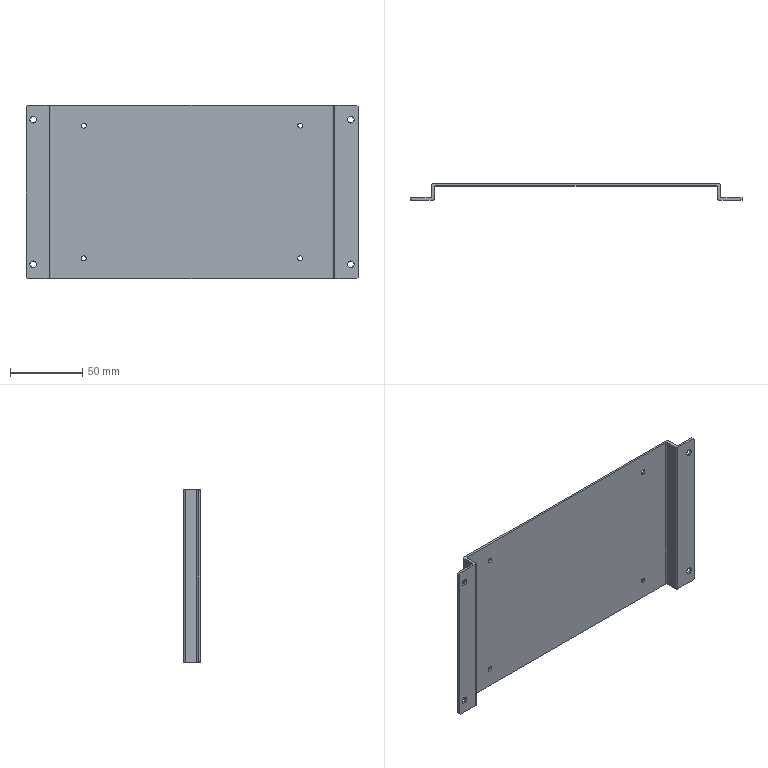Part | NX | 1 solid | 34 faces | box 230 x 11.5 x 120 mm | volume 46044 mm3 | plane 18 | cylinder 16 | commonest cylinder face diameters 2 x8 3.5 x4 4.5 x4
STEP:
#1=CARTESIAN_POINT('',(-41.764,-1.5,119.));
#2=VERTEX_POINT('',#1);
#3=CARTESIAN_POINT('',(-41.764,-1.5,1.));
#4=VERTEX_POINT('',#3);
#5=CARTESIAN_POINT('',(-41.764,-1.5,120.));
#6=DIRECTION('',(0.,0.,-1.));
#7=VECTOR('',#6,1000.);
#8=LINE('',#5,#7);
#9=EDGE_CURVE('',#2,#4,#8,.T.);
#10=ORIENTED_EDGE('',*,*,#9,.F.);
#11=CARTESIAN_POINT('',(-41.764,0.,119.));
#12=VERTEX_POINT('',#11);
#13=CARTESIAN_POINT('',(-41.764,0.,119.));
#14=DIRECTION('',(0.,1.,0.));
#15=VECTOR('',#14,1000.);
#16=LINE('',#13,#15);
#17=EDGE_CURVE('',#2,#12,#16,.T.);
#18=ORIENTED_EDGE('',*,*,#17,.T.);
#19=CARTESIAN_POINT('',(-41.764,0.,1.));
#20=VERTEX_POINT('',#19);
#21=CARTESIAN_POINT('',(-41.764,0.,120.));
#22=DIRECTION('',(0.,0.,-1.));
#23=VECTOR('',#22,1000.);
#24=LINE('',#21,#23);
#25=EDGE_CURVE('',#12,#20,#24,.T.);
#26=ORIENTED_EDGE('',*,*,#25,.T.);
#27=CARTESIAN_POINT('',(-41.764,0.,1.));
#28=DIRECTION('',(0.,-1.,0.));
#29=VECTOR('',#28,1000.);
#30=LINE('',#27,#29);
#31=EDGE_CURVE('',#20,#4,#30,.T.);
#32=ORIENTED_EDGE('',*,*,#31,.T.);
#33=EDGE_LOOP('',(#10,#18,#26,#32));
#34=FACE_BOUND('',#33,.T.);
#35=CARTESIAN_POINT('',(-41.764,0.,120.));
#36=DIRECTION('',(1.,0.,0.));
#37=DIRECTION('',(0.,0.,-1.));
#38=AXIS2_PLACEMENT_3D('',#35,#36,#37);
#39=PLANE('',#38);
#40=ADVANCED_FACE('',(#34),#39,.F.);
#41=CARTESIAN_POINT('',(-36.764,-1.5,12.25));
#42=VERTEX_POINT('',#41);
#43=CARTESIAN_POINT('',(-36.764,-1.5,10.));
#44=DIRECTION('',(0.,1.,0.));
#45=DIRECTION('',(0.,0.,1.));
#46=AXIS2_PLACEMENT_3D('',#43,#44,#45);
#47=CIRCLE('',#46,2.25);
#48=EDGE_CURVE('',#42,#42,#47,.T.);
#49=ORIENTED_EDGE('',*,*,#48,.T.);
#50=EDGE_LOOP('',(#49));
#51=FACE_BOUND('',#50,.T.);
#52=CARTESIAN_POINT('',(-36.764,-1.5,112.25));
#53=VERTEX_POINT('',#52);
#54=CARTESIAN_POINT('',(-36.764,-1.5,110.));
#55=DIRECTION('',(0.,1.,0.));
#56=DIRECTION('',(0.,0.,1.));
#57=AXIS2_PLACEMENT_3D('',#54,#55,#56);
#58=CIRCLE('',#57,2.25);
#59=EDGE_CURVE('',#53,#53,#58,.T.);
#60=ORIENTED_EDGE('',*,*,#59,.T.);
#61=EDGE_LOOP('',(#60));
#62=FACE_BOUND('',#61,.T.);
#63=CARTESIAN_POINT('',(-40.764,-1.5,120.));
#64=VERTEX_POINT('',#63);
#65=CARTESIAN_POINT('',(-25.764,-1.5,120.));
#66=VERTEX_POINT('',#65);
#67=CARTESIAN_POINT('',(-41.764,-1.5,120.));
#68=DIRECTION('',(1.,0.,0.));
#69=VECTOR('',#68,1000.);
#70=LINE('',#67,#69);
#71=EDGE_CURVE('',#64,#66,#70,.T.);
#72=ORIENTED_EDGE('',*,*,#71,.F.);
#73=CARTESIAN_POINT('',(-40.764,-1.5,120.));
#74=DIRECTION('',(-0.7071,0.,-0.7071));
#75=VECTOR('',#74,1000.);
#76=LINE('',#73,#75);
#77=EDGE_CURVE('',#64,#2,#76,.T.);
#78=ORIENTED_EDGE('',*,*,#77,.T.);
#79=ORIENTED_EDGE('',*,*,#9,.T.);
#80=CARTESIAN_POINT('',(-40.764,-1.5,0.));
#81=VERTEX_POINT('',#80);
#82=CARTESIAN_POINT('',(-41.764,-1.5,1.));
#83=DIRECTION('',(-0.7071,0.,0.7071));
#84=VECTOR('',#83,1000.);
#85=LINE('',#82,#84);
#86=EDGE_CURVE('',#4,#81,#85,.F.);
#87=ORIENTED_EDGE('',*,*,#86,.T.);
#88=CARTESIAN_POINT('',(-25.764,-1.5,0.));
#89=VERTEX_POINT('',#88);
#90=CARTESIAN_POINT('',(-41.764,-1.5,0.));
#91=DIRECTION('',(1.,0.,0.));
#92=VECTOR('',#91,1000.);
#93=LINE('',#90,#92);
#94=EDGE_CURVE('',#81,#89,#93,.T.);
#95=ORIENTED_EDGE('',*,*,#94,.T.);
#96=CARTESIAN_POINT('',(-25.764,-1.5,120.));
#97=DIRECTION('',(0.,0.,-1.));
#98=VECTOR('',#97,1000.);
#99=LINE('',#96,#98);
#100=EDGE_CURVE('',#66,#89,#99,.T.);
#101=ORIENTED_EDGE('',*,*,#100,.F.);
#102=EDGE_LOOP('',(#72,#78,#79,#87,#95,#101));
#103=FACE_BOUND('',#102,.T.);
#104=CARTESIAN_POINT('',(-41.764,-1.5,120.));
#105=DIRECTION('',(0.,1.,0.));
#106=DIRECTION('',(0.,0.,1.));
#107=AXIS2_PLACEMENT_3D('',#104,#105,#106);
#108=PLANE('',#107);
#109=ADVANCED_FACE('',(#51,#62,#103),#108,.F.);
#110=CARTESIAN_POINT('',(-24.764,-0.5,0.));
#111=VERTEX_POINT('',#110);
#112=CARTESIAN_POINT('',(-25.764,-0.5,0.));
#113=DIRECTION('',(0.,0.,1.));
#114=DIRECTION('',(1.,0.,0.));
#115=AXIS2_PLACEMENT_3D('',#112,#113,#114);
#116=CIRCLE('',#115,1.);
#117=EDGE_CURVE('',#89,#111,#116,.T.);
#118=ORIENTED_EDGE('',*,*,#117,.T.);
#119=CARTESIAN_POINT('',(-24.764,-0.5,120.));
#120=VERTEX_POINT('',#119);
#121=CARTESIAN_POINT('',(-24.764,-0.5,120.));
#122=DIRECTION('',(0.,0.,-1.));
#123=VECTOR('',#122,1000.);
#124=LINE('',#121,#123);
#125=EDGE_CURVE('',#120,#111,#124,.T.);
#126=ORIENTED_EDGE('',*,*,#125,.F.);
#127=CARTESIAN_POINT('',(-25.764,-0.5,120.));
#128=DIRECTION('',(0.,0.,1.));
#129=DIRECTION('',(1.,0.,0.));
#130=AXIS2_PLACEMENT_3D('',#127,#128,#129);
#131=CIRCLE('',#130,1.);
#132=EDGE_CURVE('',#66,#120,#131,.T.);
#133=ORIENTED_EDGE('',*,*,#132,.F.);
#134=ORIENTED_EDGE('',*,*,#100,.T.);
#135=EDGE_LOOP('',(#118,#126,#133,#134));
#136=FACE_BOUND('',#135,.T.);
#137=CARTESIAN_POINT('',(-25.764,-0.5,120.));
#138=DIRECTION('',(0.,0.,-1.));
#139=DIRECTION('',(-1.,0.,0.));
#140=AXIS2_PLACEMENT_3D('',#137,#138,#139);
#141=CYLINDRICAL_SURFACE('',#140,1.);
#142=ADVANCED_FACE('',(#136),#141,.T.);
#143=CARTESIAN_POINT('',(-24.764,7.5,0.));
#144=VERTEX_POINT('',#143);
#145=CARTESIAN_POINT('',(-24.764,-0.5,0.));
#146=DIRECTION('',(0.,1.,0.));
#147=VECTOR('',#146,1000.);
#148=LINE('',#145,#147);
#149=EDGE_CURVE('',#111,#144,#148,.T.);
#150=ORIENTED_EDGE('',*,*,#149,.T.);
#151=CARTESIAN_POINT('',(-24.764,7.5,120.));
#152=VERTEX_POINT('',#151);
#153=CARTESIAN_POINT('',(-24.764,7.5,120.));
#154=DIRECTION('',(0.,0.,-1.));
#155=VECTOR('',#154,1000.);
#156=LINE('',#153,#155);
#157=EDGE_CURVE('',#152,#144,#156,.T.);
#158=ORIENTED_EDGE('',*,*,#157,.F.);
#159=CARTESIAN_POINT('',(-24.764,-0.5,120.));
#160=DIRECTION('',(0.,1.,0.));
#161=VECTOR('',#160,1000.);
#162=LINE('',#159,#161);
#163=EDGE_CURVE('',#120,#152,#162,.T.);
#164=ORIENTED_EDGE('',*,*,#163,.F.);
#165=ORIENTED_EDGE('',*,*,#125,.T.);
#166=EDGE_LOOP('',(#150,#158,#164,#165));
#167=FACE_BOUND('',#166,.T.);
#168=CARTESIAN_POINT('',(-24.764,-0.5,120.));
#169=DIRECTION('',(-1.,0.,0.));
#170=DIRECTION('',(0.,0.,1.));
#171=AXIS2_PLACEMENT_3D('',#168,#169,#170);
#172=PLANE('',#171);
#173=ADVANCED_FACE('',(#167),#172,.F.);
#174=CARTESIAN_POINT('',(-23.764,8.5,0.));
#175=VERTEX_POINT('',#174);
#176=CARTESIAN_POINT('',(-23.764,7.5,0.));
#177=DIRECTION('',(0.,0.,-1.));
#178=DIRECTION('',(-1.,0.,0.));
#179=AXIS2_PLACEMENT_3D('',#176,#177,#178);
#180=CIRCLE('',#179,1.);
#181=EDGE_CURVE('',#144,#175,#180,.T.);
#182=ORIENTED_EDGE('',*,*,#181,.T.);
#183=CARTESIAN_POINT('',(-23.764,8.5,120.));
#184=VERTEX_POINT('',#183);
#185=CARTESIAN_POINT('',(-23.764,8.5,120.));
#186=DIRECTION('',(0.,0.,-1.));
#187=VECTOR('',#186,1000.);
#188=LINE('',#185,#187);
#189=EDGE_CURVE('',#184,#175,#188,.T.);
#190=ORIENTED_EDGE('',*,*,#189,.F.);
#191=CARTESIAN_POINT('',(-23.764,7.5,120.));
#192=DIRECTION('',(0.,0.,-1.));
#193=DIRECTION('',(-1.,0.,0.));
#194=AXIS2_PLACEMENT_3D('',#191,#192,#193);
#195=CIRCLE('',#194,1.);
#196=EDGE_CURVE('',#152,#184,#195,.T.);
#197=ORIENTED_EDGE('',*,*,#196,.F.);
#198=ORIENTED_EDGE('',*,*,#157,.T.);
#199=EDGE_LOOP('',(#182,#190,#197,#198));
#200=FACE_BOUND('',#199,.T.);
#201=CARTESIAN_POINT('',(-23.764,7.5,120.));
#202=DIRECTION('',(0.,0.,-1.));
#203=DIRECTION('',(-1.,0.,0.));
#204=AXIS2_PLACEMENT_3D('',#201,#202,#203);
#205=CYLINDRICAL_SURFACE('',#204,1.);
#206=ADVANCED_FACE('',(#200),#205,.F.);
#207=CARTESIAN_POINT('',(-3.514,8.5,14.));
#208=VERTEX_POINT('',#207);
#209=CARTESIAN_POINT('',(-1.764,8.5,14.));
#210=DIRECTION('',(0.,1.,0.));
#211=DIRECTION('',(-1.,0.,0.));
#212=AXIS2_PLACEMENT_3D('',#209,#210,#211);
#213=CIRCLE('',#212,1.75);
#214=EDGE_CURVE('',#208,#208,#213,.T.);
#215=ORIENTED_EDGE('',*,*,#214,.T.);
#216=EDGE_LOOP('',(#215));
#217=FACE_BOUND('',#216,.T.);
#218=CARTESIAN_POINT('',(-3.514,8.5,106.));
#219=VERTEX_POINT('',#218);
#220=CARTESIAN_POINT('',(-1.764,8.5,106.));
#221=DIRECTION('',(0.,1.,0.));
#222=DIRECTION('',(-1.,0.,0.));
#223=AXIS2_PLACEMENT_3D('',#220,#221,#222);
#224=CIRCLE('',#223,1.75);
#225=EDGE_CURVE('',#219,#219,#224,.T.);
#226=ORIENTED_EDGE('',*,*,#225,.T.);
#227=EDGE_LOOP('',(#226));
#228=FACE_BOUND('',#227,.T.);
#229=CARTESIAN_POINT('',(146.486,8.5,106.));
#230=VERTEX_POINT('',#229);
#231=CARTESIAN_POINT('',(148.236,8.5,106.));
#232=DIRECTION('',(0.,1.,0.));
#233=DIRECTION('',(-1.,0.,0.));
#234=AXIS2_PLACEMENT_3D('',#231,#232,#233);
#235=CIRCLE('',#234,1.75);
#236=EDGE_CURVE('',#230,#230,#235,.T.);
#237=ORIENTED_EDGE('',*,*,#236,.T.);
#238=EDGE_LOOP('',(#237));
#239=FACE_BOUND('',#238,.T.);
#240=CARTESIAN_POINT('',(146.486,8.5,14.));
#241=VERTEX_POINT('',#240);
#242=CARTESIAN_POINT('',(148.236,8.5,14.));
#243=DIRECTION('',(0.,1.,0.));
#244=DIRECTION('',(-1.,0.,0.));
#245=AXIS2_PLACEMENT_3D('',#242,#243,#244);
#246=CIRCLE('',#245,1.75);
#247=EDGE_CURVE('',#241,#241,#246,.T.);
#248=ORIENTED_EDGE('',*,*,#247,.T.);
#249=EDGE_LOOP('',(#248));
#250=FACE_BOUND('',#249,.T.);
#251=CARTESIAN_POINT('',(170.236,8.5,0.));
#252=VERTEX_POINT('',#251);
#253=CARTESIAN_POINT('',(-23.764,8.5,0.));
#254=DIRECTION('',(1.,0.,0.));
#255=VECTOR('',#254,1000.);
#256=LINE('',#253,#255);
#257=EDGE_CURVE('',#175,#252,#256,.T.);
#258=ORIENTED_EDGE('',*,*,#257,.T.);
#259=CARTESIAN_POINT('',(170.236,8.5,120.));
#260=VERTEX_POINT('',#259);
#261=CARTESIAN_POINT('',(170.236,8.5,120.));
#262=DIRECTION('',(0.,0.,-1.));
#263=VECTOR('',#262,1000.);
#264=LINE('',#261,#263);
#265=EDGE_CURVE('',#260,#252,#264,.T.);
#266=ORIENTED_EDGE('',*,*,#265,.F.);
#267=CARTESIAN_POINT('',(-23.764,8.5,120.));
#268=DIRECTION('',(1.,0.,0.));
#269=VECTOR('',#268,1000.);
#270=LINE('',#267,#269);
#271=EDGE_CURVE('',#184,#260,#270,.T.);
#272=ORIENTED_EDGE('',*,*,#271,.F.);
#273=ORIENTED_EDGE('',*,*,#189,.T.);
#274=EDGE_LOOP('',(#258,#266,#272,#273));
#275=FACE_BOUND('',#274,.T.);
#276=CARTESIAN_POINT('',(-23.764,8.5,120.));
#277=DIRECTION('',(0.,1.,0.));
#278=DIRECTION('',(-1.,0.,0.));
#279=AXIS2_PLACEMENT_3D('',#276,#277,#278);
#280=PLANE('',#279);
#281=ADVANCED_FACE('',(#217,#228,#239,#250,#275),#280,.F.);
#282=CARTESIAN_POINT('',(171.236,7.5,0.));
#283=VERTEX_POINT('',#282);
#284=CARTESIAN_POINT('',(170.236,7.5,0.));
#285=DIRECTION('',(0.,0.,-1.));
#286=DIRECTION('',(-1.,0.,0.));
#287=AXIS2_PLACEMENT_3D('',#284,#285,#286);
#288=CIRCLE('',#287,1.);
#289=EDGE_CURVE('',#252,#283,#288,.T.);
#290=ORIENTED_EDGE('',*,*,#289,.T.);
#291=CARTESIAN_POINT('',(171.236,7.5,120.));
#292=VERTEX_POINT('',#291);
#293=CARTESIAN_POINT('',(171.236,7.5,120.));
#294=DIRECTION('',(0.,0.,-1.));
#295=VECTOR('',#294,1000.);
#296=LINE('',#293,#295);
#297=EDGE_CURVE('',#292,#283,#296,.T.);
#298=ORIENTED_EDGE('',*,*,#297,.F.);
#299=CARTESIAN_POINT('',(170.236,7.5,120.));
#300=DIRECTION('',(0.,0.,-1.));
#301=DIRECTION('',(-1.,0.,0.));
#302=AXIS2_PLACEMENT_3D('',#299,#300,#301);
#303=CIRCLE('',#302,1.);
#304=EDGE_CURVE('',#260,#292,#303,.T.);
#305=ORIENTED_EDGE('',*,*,#304,.F.);
#306=ORIENTED_EDGE('',*,*,#265,.T.);
#307=EDGE_LOOP('',(#290,#298,#305,#306));
#308=FACE_BOUND('',#307,.T.);
#309=CARTESIAN_POINT('',(170.236,7.5,120.));
#310=DIRECTION('',(0.,0.,-1.));
#311=DIRECTION('',(-1.,0.,0.));
#312=AXIS2_PLACEMENT_3D('',#309,#310,#311);
#313=CYLINDRICAL_SURFACE('',#312,1.);
#314=ADVANCED_FACE('',(#308),#313,.F.);
#315=CARTESIAN_POINT('',(171.236,-0.5,0.));
#316=VERTEX_POINT('',#315);
#317=CARTESIAN_POINT('',(171.236,7.5,0.));
#318=DIRECTION('',(0.,-1.,0.));
#319=VECTOR('',#318,1000.);
#320=LINE('',#317,#319);
#321=EDGE_CURVE('',#283,#316,#320,.T.);
#322=ORIENTED_EDGE('',*,*,#321,.T.);
#323=CARTESIAN_POINT('',(171.236,-0.5,120.));
#324=VERTEX_POINT('',#323);
#325=CARTESIAN_POINT('',(171.236,-0.5,120.));
#326=DIRECTION('',(0.,0.,-1.));
#327=VECTOR('',#326,1000.);
#328=LINE('',#325,#327);
#329=EDGE_CURVE('',#324,#316,#328,.T.);
#330=ORIENTED_EDGE('',*,*,#329,.F.);
#331=CARTESIAN_POINT('',(171.236,7.5,120.));
#332=DIRECTION('',(0.,-1.,0.));
#333=VECTOR('',#332,1000.);
#334=LINE('',#331,#333);
#335=EDGE_CURVE('',#292,#324,#334,.T.);
#336=ORIENTED_EDGE('',*,*,#335,.F.);
#337=ORIENTED_EDGE('',*,*,#297,.T.);
#338=EDGE_LOOP('',(#322,#330,#336,#337));
#339=FACE_BOUND('',#338,.T.);
#340=CARTESIAN_POINT('',(171.236,7.5,120.));
#341=DIRECTION('',(1.,0.,0.));
#342=DIRECTION('',(0.,0.,-1.));
#343=AXIS2_PLACEMENT_3D('',#340,#341,#342);
#344=PLANE('',#343);
#345=ADVANCED_FACE('',(#339),#344,.F.);
#346=CARTESIAN_POINT('',(172.236,-1.5,0.));
#347=VERTEX_POINT('',#346);
#348=CARTESIAN_POINT('',(172.236,-0.5,0.));
#349=DIRECTION('',(0.,0.,1.));
#350=DIRECTION('',(1.,0.,0.));
#351=AXIS2_PLACEMENT_3D('',#348,#349,#350);
#352=CIRCLE('',#351,1.);
#353=EDGE_CURVE('',#316,#347,#352,.T.);
#354=ORIENTED_EDGE('',*,*,#353,.T.);
#355=CARTESIAN_POINT('',(172.236,-1.5,120.));
#356=VERTEX_POINT('',#355);
#357=CARTESIAN_POINT('',(172.236,-1.5,120.));
#358=DIRECTION('',(0.,0.,-1.));
#359=VECTOR('',#358,1000.);
#360=LINE('',#357,#359);
#361=EDGE_CURVE('',#356,#347,#360,.T.);
#362=ORIENTED_EDGE('',*,*,#361,.F.);
#363=CARTESIAN_POINT('',(172.236,-0.5,120.));
#364=DIRECTION('',(0.,0.,1.));
#365=DIRECTION('',(1.,0.,0.));
#366=AXIS2_PLACEMENT_3D('',#363,#364,#365);
#367=CIRCLE('',#366,1.);
#368=EDGE_CURVE('',#324,#356,#367,.T.);
#369=ORIENTED_EDGE('',*,*,#368,.F.);
#370=ORIENTED_EDGE('',*,*,#329,.T.);
#371=EDGE_LOOP('',(#354,#362,#369,#370));
#372=FACE_BOUND('',#371,.T.);
#373=CARTESIAN_POINT('',(172.236,-0.5,120.));
#374=DIRECTION('',(0.,0.,-1.));
#375=DIRECTION('',(-1.,0.,0.));
#376=AXIS2_PLACEMENT_3D('',#373,#374,#375);
#377=CYLINDRICAL_SURFACE('',#376,1.);
#378=ADVANCED_FACE('',(#372),#377,.T.);
#379=CARTESIAN_POINT('',(183.236,-1.5,112.25));
#380=VERTEX_POINT('',#379);
#381=CARTESIAN_POINT('',(183.236,-1.5,110.));
#382=DIRECTION('',(0.,1.,0.));
#383=DIRECTION('',(0.,0.,1.));
#384=AXIS2_PLACEMENT_3D('',#381,#382,#383);
#385=CIRCLE('',#384,2.25);
#386=EDGE_CURVE('',#380,#380,#385,.T.);
#387=ORIENTED_EDGE('',*,*,#386,.T.);
#388=EDGE_LOOP('',(#387));
#389=FACE_BOUND('',#388,.T.);
#390=CARTESIAN_POINT('',(183.236,-1.5,12.25));
#391=VERTEX_POINT('',#390);
#392=CARTESIAN_POINT('',(183.236,-1.5,10.));
#393=DIRECTION('',(0.,1.,0.));
#394=DIRECTION('',(0.,0.,1.));
#395=AXIS2_PLACEMENT_3D('',#392,#393,#394);
#396=CIRCLE('',#395,2.25);
#397=EDGE_CURVE('',#391,#391,#396,.T.);
#398=ORIENTED_EDGE('',*,*,#397,.T.);
#399=EDGE_LOOP('',(#398));
#400=FACE_BOUND('',#399,.T.);
#401=CARTESIAN_POINT('',(187.236,-1.5,0.));
#402=VERTEX_POINT('',#401);
#403=CARTESIAN_POINT('',(172.236,-1.5,0.));
#404=DIRECTION('',(1.,0.,0.));
#405=VECTOR('',#404,1000.);
#406=LINE('',#403,#405);
#407=EDGE_CURVE('',#347,#402,#406,.T.);
#408=ORIENTED_EDGE('',*,*,#407,.T.);
#409=CARTESIAN_POINT('',(188.236,-1.5,1.));
#410=VERTEX_POINT('',#409);
#411=CARTESIAN_POINT('',(188.236,-1.5,1.));
#412=DIRECTION('',(-0.7071,0.,-0.7071));
#413=VECTOR('',#412,1000.);
#414=LINE('',#411,#413);
#415=EDGE_CURVE('',#402,#410,#414,.F.);
#416=ORIENTED_EDGE('',*,*,#415,.T.);
#417=CARTESIAN_POINT('',(188.236,-1.5,119.));
#418=VERTEX_POINT('',#417);
#419=CARTESIAN_POINT('',(188.236,-1.5,120.));
#420=DIRECTION('',(0.,0.,-1.));
#421=VECTOR('',#420,1000.);
#422=LINE('',#419,#421);
#423=EDGE_CURVE('',#418,#410,#422,.T.);
#424=ORIENTED_EDGE('',*,*,#423,.F.);
#425=CARTESIAN_POINT('',(187.236,-1.5,120.));
#426=VERTEX_POINT('',#425);
#427=CARTESIAN_POINT('',(187.236,-1.5,120.));
#428=DIRECTION('',(-0.7071,0.,0.7071));
#429=VECTOR('',#428,1000.);
#430=LINE('',#427,#429);
#431=EDGE_CURVE('',#418,#426,#430,.T.);
#432=ORIENTED_EDGE('',*,*,#431,.T.);
#433=CARTESIAN_POINT('',(172.236,-1.5,120.));
#434=DIRECTION('',(1.,0.,0.));
#435=VECTOR('',#434,1000.);
#436=LINE('',#433,#435);
#437=EDGE_CURVE('',#356,#426,#436,.T.);
#438=ORIENTED_EDGE('',*,*,#437,.F.);
#439=ORIENTED_EDGE('',*,*,#361,.T.);
#440=EDGE_LOOP('',(#408,#416,#424,#432,#438,#439));
#441=FACE_BOUND('',#440,.T.);
#442=CARTESIAN_POINT('',(172.236,-1.5,120.));
#443=DIRECTION('',(0.,1.,0.));
#444=DIRECTION('',(0.,0.,1.));
#445=AXIS2_PLACEMENT_3D('',#442,#443,#444);
#446=PLANE('',#445);
#447=ADVANCED_FACE('',(#389,#400,#441),#446,.F.);
#448=ORIENTED_EDGE('',*,*,#423,.T.);
#449=CARTESIAN_POINT('',(188.236,0.,1.));
#450=VERTEX_POINT('',#449);
#451=CARTESIAN_POINT('',(188.236,-1.5,1.));
#452=DIRECTION('',(0.,1.,0.));
#453=VECTOR('',#452,1000.);
#454=LINE('',#451,#453);
#455=EDGE_CURVE('',#410,#450,#454,.T.);
#456=ORIENTED_EDGE('',*,*,#455,.T.);
#457=CARTESIAN_POINT('',(188.236,0.,119.));
#458=VERTEX_POINT('',#457);
#459=CARTESIAN_POINT('',(188.236,0.,120.));
#460=DIRECTION('',(0.,0.,-1.));
#461=VECTOR('',#460,1000.);
#462=LINE('',#459,#461);
#463=EDGE_CURVE('',#458,#450,#462,.T.);
#464=ORIENTED_EDGE('',*,*,#463,.F.);
#465=CARTESIAN_POINT('',(188.236,-1.5,119.));
#466=DIRECTION('',(0.,-1.,0.));
#467=VECTOR('',#466,1000.);
#468=LINE('',#465,#467);
#469=EDGE_CURVE('',#458,#418,#468,.T.);
#470=ORIENTED_EDGE('',*,*,#469,.T.);
#471=EDGE_LOOP('',(#448,#456,#464,#470));
#472=FACE_BOUND('',#471,.T.);
#473=CARTESIAN_POINT('',(188.236,-1.5,120.));
#474=DIRECTION('',(-1.,0.,0.));
#475=DIRECTION('',(0.,0.,1.));
#476=AXIS2_PLACEMENT_3D('',#473,#474,#475);
#477=PLANE('',#476);
#478=ADVANCED_FACE('',(#472),#477,.F.);
#479=CARTESIAN_POINT('',(183.236,0.,112.25));
#480=VERTEX_POINT('',#479);
#481=CARTESIAN_POINT('',(183.236,0.,110.));
#482=DIRECTION('',(0.,1.,0.));
#483=DIRECTION('',(0.,0.,1.));
#484=AXIS2_PLACEMENT_3D('',#481,#482,#483);
#485=CIRCLE('',#484,2.25);
#486=EDGE_CURVE('',#480,#480,#485,.T.);
#487=ORIENTED_EDGE('',*,*,#486,.F.);
#488=EDGE_LOOP('',(#487));
#489=FACE_BOUND('',#488,.T.);
#490=CARTESIAN_POINT('',(183.236,0.,12.25));
#491=VERTEX_POINT('',#490);
#492=CARTESIAN_POINT('',(183.236,0.,10.));
#493=DIRECTION('',(0.,1.,0.));
#494=DIRECTION('',(0.,0.,1.));
#495=AXIS2_PLACEMENT_3D('',#492,#493,#494);
#496=CIRCLE('',#495,2.25);
#497=EDGE_CURVE('',#491,#491,#496,.T.);
#498=ORIENTED_EDGE('',*,*,#497,.F.);
#499=EDGE_LOOP('',(#498));
#500=FACE_BOUND('',#499,.T.);
#501=ORIENTED_EDGE('',*,*,#463,.T.);
#502=CARTESIAN_POINT('',(187.236,0.,0.));
#503=VERTEX_POINT('',#502);
#504=CARTESIAN_POINT('',(188.236,0.,1.));
#505=DIRECTION('',(0.7071,0.,0.7071));
#506=VECTOR('',#505,1000.);
#507=LINE('',#504,#506);
#508=EDGE_CURVE('',#450,#503,#507,.F.);
#509=ORIENTED_EDGE('',*,*,#508,.T.);
#510=CARTESIAN_POINT('',(174.236,0.,0.));
#511=VERTEX_POINT('',#510);
#512=CARTESIAN_POINT('',(174.236,0.,0.));
#513=DIRECTION('',(-1.,0.,0.));
#514=VECTOR('',#513,1000.);
#515=LINE('',#512,#514);
#516=EDGE_CURVE('',#503,#511,#515,.T.);
#517=ORIENTED_EDGE('',*,*,#516,.T.);
#518=CARTESIAN_POINT('',(174.236,0.,120.));
#519=VERTEX_POINT('',#518);
#520=CARTESIAN_POINT('',(174.236,0.,120.));
#521=DIRECTION('',(0.,0.,-1.));
#522=VECTOR('',#521,1000.);
#523=LINE('',#520,#522);
#524=EDGE_CURVE('',#519,#511,#523,.T.);
#525=ORIENTED_EDGE('',*,*,#524,.F.);
#526=CARTESIAN_POINT('',(187.236,0.,120.));
#527=VERTEX_POINT('',#526);
#528=CARTESIAN_POINT('',(174.236,0.,120.));
#529=DIRECTION('',(-1.,0.,0.));
#530=VECTOR('',#529,1000.);
#531=LINE('',#528,#530);
#532=EDGE_CURVE('',#527,#519,#531,.T.);
#533=ORIENTED_EDGE('',*,*,#532,.F.);
#534=CARTESIAN_POINT('',(187.236,0.,120.));
#535=DIRECTION('',(0.7071,0.,-0.7071));
#536=VECTOR('',#535,1000.);
#537=LINE('',#534,#536);
#538=EDGE_CURVE('',#527,#458,#537,.T.);
#539=ORIENTED_EDGE('',*,*,#538,.T.);
#540=EDGE_LOOP('',(#501,#509,#517,#525,#533,#539));
#541=FACE_BOUND('',#540,.T.);
#542=CARTESIAN_POINT('',(174.236,0.,120.));
#543=DIRECTION('',(0.,-1.,0.));
#544=DIRECTION('',(0.,0.,-1.));
#545=AXIS2_PLACEMENT_3D('',#542,#543,#544);
#546=PLANE('',#545);
#547=ADVANCED_FACE('',(#489,#500,#541),#546,.F.);
#548=CARTESIAN_POINT('',(173.236,1.,0.));
#549=VERTEX_POINT('',#548);
#550=CARTESIAN_POINT('',(174.236,1.,0.));
#551=DIRECTION('',(0.,0.,-1.));
#552=DIRECTION('',(1.,0.,0.));
#553=AXIS2_PLACEMENT_3D('',#550,#551,#552);
#554=CIRCLE('',#553,1.);
#555=EDGE_CURVE('',#511,#549,#554,.T.);
#556=ORIENTED_EDGE('',*,*,#555,.T.);
#557=CARTESIAN_POINT('',(173.236,1.,120.));
#558=VERTEX_POINT('',#557);
#559=CARTESIAN_POINT('',(173.236,1.,120.));
#560=DIRECTION('',(0.,0.,-1.));
#561=VECTOR('',#560,1000.);
#562=LINE('',#559,#561);
#563=EDGE_CURVE('',#558,#549,#562,.T.);
#564=ORIENTED_EDGE('',*,*,#563,.F.);
#565=CARTESIAN_POINT('',(174.236,1.,120.));
#566=DIRECTION('',(0.,0.,-1.));
#567=DIRECTION('',(1.,0.,0.));
#568=AXIS2_PLACEMENT_3D('',#565,#566,#567);
#569=CIRCLE('',#568,1.);
#570=EDGE_CURVE('',#519,#558,#569,.T.);
#571=ORIENTED_EDGE('',*,*,#570,.F.);
#572=ORIENTED_EDGE('',*,*,#524,.T.);
#573=EDGE_LOOP('',(#556,#564,#571,#572));
#574=FACE_BOUND('',#573,.T.);
#575=CARTESIAN_POINT('',(174.236,1.,120.));
#576=DIRECTION('',(0.,0.,-1.));
#577=DIRECTION('',(-1.,0.,0.));
#578=AXIS2_PLACEMENT_3D('',#575,#576,#577);
#579=CYLINDRICAL_SURFACE('',#578,1.);
#580=ADVANCED_FACE('',(#574),#579,.F.);
#581=CARTESIAN_POINT('',(173.236,9.,0.));
#582=VERTEX_POINT('',#581);
#583=CARTESIAN_POINT('',(173.236,9.,0.));
#584=DIRECTION('',(0.,1.,0.));
#585=VECTOR('',#584,1000.);
#586=LINE('',#583,#585);
#587=EDGE_CURVE('',#549,#582,#586,.T.);
#588=ORIENTED_EDGE('',*,*,#587,.T.);
#589=CARTESIAN_POINT('',(173.236,9.,120.));
#590=VERTEX_POINT('',#589);
#591=CARTESIAN_POINT('',(173.236,9.,120.));
#592=DIRECTION('',(0.,0.,-1.));
#593=VECTOR('',#592,1000.);
#594=LINE('',#591,#593);
#595=EDGE_CURVE('',#590,#582,#594,.T.);
#596=ORIENTED_EDGE('',*,*,#595,.F.);
#597=CARTESIAN_POINT('',(173.236,9.,120.));
#598=DIRECTION('',(0.,1.,0.));
#599=VECTOR('',#598,1000.);
#600=LINE('',#597,#599);
#601=EDGE_CURVE('',#558,#590,#600,.T.);
#602=ORIENTED_EDGE('',*,*,#601,.F.);
#603=ORIENTED_EDGE('',*,*,#563,.T.);
#604=EDGE_LOOP('',(#588,#596,#602,#603));
#605=FACE_BOUND('',#604,.T.);
#606=CARTESIAN_POINT('',(173.236,9.,120.));
#607=DIRECTION('',(-1.,0.,0.));
#608=DIRECTION('',(0.,0.,1.));
#609=AXIS2_PLACEMENT_3D('',#606,#607,#608);
#610=PLANE('',#609);
#611=ADVANCED_FACE('',(#605),#610,.F.);
#612=CARTESIAN_POINT('',(172.236,10.,0.));
#613=VERTEX_POINT('',#612);
#614=CARTESIAN_POINT('',(172.236,9.,0.));
#615=DIRECTION('',(0.,0.,1.));
#616=DIRECTION('',(-1.,0.,0.));
#617=AXIS2_PLACEMENT_3D('',#614,#615,#616);
#618=CIRCLE('',#617,1.);
#619=EDGE_CURVE('',#582,#613,#618,.T.);
#620=ORIENTED_EDGE('',*,*,#619,.T.);
#621=CARTESIAN_POINT('',(172.236,10.,120.));
#622=VERTEX_POINT('',#621);
#623=CARTESIAN_POINT('',(172.236,10.,120.));
#624=DIRECTION('',(0.,0.,-1.));
#625=VECTOR('',#624,1000.);
#626=LINE('',#623,#625);
#627=EDGE_CURVE('',#622,#613,#626,.T.);
#628=ORIENTED_EDGE('',*,*,#627,.F.);
#629=CARTESIAN_POINT('',(172.236,9.,120.));
#630=DIRECTION('',(0.,0.,1.));
#631=DIRECTION('',(-1.,0.,0.));
#632=AXIS2_PLACEMENT_3D('',#629,#630,#631);
#633=CIRCLE('',#632,1.);
#634=EDGE_CURVE('',#590,#622,#633,.T.);
#635=ORIENTED_EDGE('',*,*,#634,.F.);
#636=ORIENTED_EDGE('',*,*,#595,.T.);
#637=EDGE_LOOP('',(#620,#628,#635,#636));
#638=FACE_BOUND('',#637,.T.);
#639=CARTESIAN_POINT('',(172.236,9.,120.));
#640=DIRECTION('',(0.,0.,-1.));
#641=DIRECTION('',(-1.,0.,0.));
#642=AXIS2_PLACEMENT_3D('',#639,#640,#641);
#643=CYLINDRICAL_SURFACE('',#642,1.);
#644=ADVANCED_FACE('',(#638),#643,.T.);
#645=CARTESIAN_POINT('',(-1.764,10.,15.75));
#646=VERTEX_POINT('',#645);
#647=CARTESIAN_POINT('',(-1.764,10.,14.));
#648=DIRECTION('',(0.,1.,0.));
#649=DIRECTION('',(0.,0.,1.));
#650=AXIS2_PLACEMENT_3D('',#647,#648,#649);
#651=CIRCLE('',#650,1.75);
#652=EDGE_CURVE('',#646,#646,#651,.T.);
#653=ORIENTED_EDGE('',*,*,#652,.F.);
#654=EDGE_LOOP('',(#653));
#655=FACE_BOUND('',#654,.T.);
#656=CARTESIAN_POINT('',(-1.764,10.,107.75));
#657=VERTEX_POINT('',#656);
#658=CARTESIAN_POINT('',(-1.764,10.,106.));
#659=DIRECTION('',(0.,1.,0.));
#660=DIRECTION('',(0.,0.,1.));
#661=AXIS2_PLACEMENT_3D('',#658,#659,#660);
#662=CIRCLE('',#661,1.75);
#663=EDGE_CURVE('',#657,#657,#662,.T.);
#664=ORIENTED_EDGE('',*,*,#663,.F.);
#665=EDGE_LOOP('',(#664));
#666=FACE_BOUND('',#665,.T.);
#667=CARTESIAN_POINT('',(148.236,10.,107.75));
#668=VERTEX_POINT('',#667);
#669=CARTESIAN_POINT('',(148.236,10.,106.));
#670=DIRECTION('',(0.,1.,0.));
#671=DIRECTION('',(0.,0.,1.));
#672=AXIS2_PLACEMENT_3D('',#669,#670,#671);
#673=CIRCLE('',#672,1.75);
#674=EDGE_CURVE('',#668,#668,#673,.T.);
#675=ORIENTED_EDGE('',*,*,#674,.F.);
#676=EDGE_LOOP('',(#675));
#677=FACE_BOUND('',#676,.T.);
#678=CARTESIAN_POINT('',(148.236,10.,15.75));
#679=VERTEX_POINT('',#678);
#680=CARTESIAN_POINT('',(148.236,10.,14.));
#681=DIRECTION('',(0.,1.,0.));
#682=DIRECTION('',(0.,0.,1.));
#683=AXIS2_PLACEMENT_3D('',#680,#681,#682);
#684=CIRCLE('',#683,1.75);
#685=EDGE_CURVE('',#679,#679,#684,.T.);
#686=ORIENTED_EDGE('',*,*,#685,.F.);
#687=EDGE_LOOP('',(#686));
#688=FACE_BOUND('',#687,.T.);
#689=CARTESIAN_POINT('',(-25.764,10.,0.));
#690=VERTEX_POINT('',#689);
#691=CARTESIAN_POINT('',(-25.764,10.,0.));
#692=DIRECTION('',(-1.,0.,0.));
#693=VECTOR('',#692,1000.);
#694=LINE('',#691,#693);
#695=EDGE_CURVE('',#613,#690,#694,.T.);
#696=ORIENTED_EDGE('',*,*,#695,.T.);
#697=CARTESIAN_POINT('',(-25.764,10.,120.));
#698=VERTEX_POINT('',#697);
#699=CARTESIAN_POINT('',(-25.764,10.,120.));
#700=DIRECTION('',(0.,0.,-1.));
#701=VECTOR('',#700,1000.);
#702=LINE('',#699,#701);
#703=EDGE_CURVE('',#698,#690,#702,.T.);
#704=ORIENTED_EDGE('',*,*,#703,.F.);
#705=CARTESIAN_POINT('',(-25.764,10.,120.));
#706=DIRECTION('',(-1.,0.,0.));
#707=VECTOR('',#706,1000.);
#708=LINE('',#705,#707);
#709=EDGE_CURVE('',#622,#698,#708,.T.);
#710=ORIENTED_EDGE('',*,*,#709,.F.);
#711=ORIENTED_EDGE('',*,*,#627,.T.);
#712=EDGE_LOOP('',(#696,#704,#710,#711));
#713=FACE_BOUND('',#712,.T.);
#714=CARTESIAN_POINT('',(-25.764,10.,120.));
#715=DIRECTION('',(0.,-1.,0.));
#716=DIRECTION('',(0.,0.,-1.));
#717=AXIS2_PLACEMENT_3D('',#714,#715,#716);
#718=PLANE('',#717);
#719=ADVANCED_FACE('',(#655,#666,#677,#688,#713),#718,.F.);
#720=CARTESIAN_POINT('',(-26.764,9.,0.));
#721=VERTEX_POINT('',#720);
#722=CARTESIAN_POINT('',(-25.764,9.,0.));
#723=DIRECTION('',(0.,0.,1.));
#724=DIRECTION('',(-1.,0.,0.));
#725=AXIS2_PLACEMENT_3D('',#722,#723,#724);
#726=CIRCLE('',#725,1.);
#727=EDGE_CURVE('',#690,#721,#726,.T.);
#728=ORIENTED_EDGE('',*,*,#727,.T.);
#729=CARTESIAN_POINT('',(-26.764,9.,120.));
#730=VERTEX_POINT('',#729);
#731=CARTESIAN_POINT('',(-26.764,9.,120.));
#732=DIRECTION('',(0.,0.,-1.));
#733=VECTOR('',#732,1000.);
#734=LINE('',#731,#733);
#735=EDGE_CURVE('',#730,#721,#734,.T.);
#736=ORIENTED_EDGE('',*,*,#735,.F.);
#737=CARTESIAN_POINT('',(-25.764,9.,120.));
#738=DIRECTION('',(0.,0.,1.));
#739=DIRECTION('',(-1.,0.,0.));
#740=AXIS2_PLACEMENT_3D('',#737,#738,#739);
#741=CIRCLE('',#740,1.);
#742=EDGE_CURVE('',#698,#730,#741,.T.);
#743=ORIENTED_EDGE('',*,*,#742,.F.);
#744=ORIENTED_EDGE('',*,*,#703,.T.);
#745=EDGE_LOOP('',(#728,#736,#743,#744));
#746=FACE_BOUND('',#745,.T.);
#747=CARTESIAN_POINT('',(-25.764,9.,120.));
#748=DIRECTION('',(0.,0.,-1.));
#749=DIRECTION('',(-1.,0.,0.));
#750=AXIS2_PLACEMENT_3D('',#747,#748,#749);
#751=CYLINDRICAL_SURFACE('',#750,1.);
#752=ADVANCED_FACE('',(#746),#751,.T.);
#753=CARTESIAN_POINT('',(-26.764,1.,0.));
#754=VERTEX_POINT('',#753);
#755=CARTESIAN_POINT('',(-26.764,1.,0.));
#756=DIRECTION('',(0.,-1.,0.));
#757=VECTOR('',#756,1000.);
#758=LINE('',#755,#757);
#759=EDGE_CURVE('',#721,#754,#758,.T.);
#760=ORIENTED_EDGE('',*,*,#759,.T.);
#761=CARTESIAN_POINT('',(-26.764,1.,120.));
#762=VERTEX_POINT('',#761);
#763=CARTESIAN_POINT('',(-26.764,1.,120.));
#764=DIRECTION('',(0.,0.,-1.));
#765=VECTOR('',#764,1000.);
#766=LINE('',#763,#765);
#767=EDGE_CURVE('',#762,#754,#766,.T.);
#768=ORIENTED_EDGE('',*,*,#767,.F.);
#769=CARTESIAN_POINT('',(-26.764,1.,120.));
#770=DIRECTION('',(0.,-1.,0.));
#771=VECTOR('',#770,1000.);
#772=LINE('',#769,#771);
#773=EDGE_CURVE('',#730,#762,#772,.T.);
#774=ORIENTED_EDGE('',*,*,#773,.F.);
#775=ORIENTED_EDGE('',*,*,#735,.T.);
#776=EDGE_LOOP('',(#760,#768,#774,#775));
#777=FACE_BOUND('',#776,.T.);
#778=CARTESIAN_POINT('',(-26.764,1.,120.));
#779=DIRECTION('',(1.,0.,0.));
#780=DIRECTION('',(0.,0.,-1.));
#781=AXIS2_PLACEMENT_3D('',#778,#779,#780);
#782=PLANE('',#781);
#783=ADVANCED_FACE('',(#777),#782,.F.);
#784=CARTESIAN_POINT('',(-27.764,0.,0.));
#785=VERTEX_POINT('',#784);
#786=CARTESIAN_POINT('',(-27.764,1.,0.));
#787=DIRECTION('',(0.,0.,-1.));
#788=DIRECTION('',(1.,0.,0.));
#789=AXIS2_PLACEMENT_3D('',#786,#787,#788);
#790=CIRCLE('',#789,1.);
#791=EDGE_CURVE('',#754,#785,#790,.T.);
#792=ORIENTED_EDGE('',*,*,#791,.T.);
#793=CARTESIAN_POINT('',(-27.764,0.,120.));
#794=VERTEX_POINT('',#793);
#795=CARTESIAN_POINT('',(-27.764,0.,120.));
#796=DIRECTION('',(0.,0.,-1.));
#797=VECTOR('',#796,1000.);
#798=LINE('',#795,#797);
#799=EDGE_CURVE('',#794,#785,#798,.T.);
#800=ORIENTED_EDGE('',*,*,#799,.F.);
#801=CARTESIAN_POINT('',(-27.764,1.,120.));
#802=DIRECTION('',(0.,0.,-1.));
#803=DIRECTION('',(1.,0.,0.));
#804=AXIS2_PLACEMENT_3D('',#801,#802,#803);
#805=CIRCLE('',#804,1.);
#806=EDGE_CURVE('',#762,#794,#805,.T.);
#807=ORIENTED_EDGE('',*,*,#806,.F.);
#808=ORIENTED_EDGE('',*,*,#767,.T.);
#809=EDGE_LOOP('',(#792,#800,#807,#808));
#810=FACE_BOUND('',#809,.T.);
#811=CARTESIAN_POINT('',(-27.764,1.,120.));
#812=DIRECTION('',(0.,0.,-1.));
#813=DIRECTION('',(-1.,0.,0.));
#814=AXIS2_PLACEMENT_3D('',#811,#812,#813);
#815=CYLINDRICAL_SURFACE('',#814,1.);
#816=ADVANCED_FACE('',(#810),#815,.F.);
#817=CARTESIAN_POINT('',(-36.764,0.,12.25));
#818=VERTEX_POINT('',#817);
#819=CARTESIAN_POINT('',(-36.764,0.,10.));
#820=DIRECTION('',(0.,1.,0.));
#821=DIRECTION('',(0.,0.,1.));
#822=AXIS2_PLACEMENT_3D('',#819,#820,#821);
#823=CIRCLE('',#822,2.25);
#824=EDGE_CURVE('',#818,#818,#823,.T.);
#825=ORIENTED_EDGE('',*,*,#824,.F.);
#826=EDGE_LOOP('',(#825));
#827=FACE_BOUND('',#826,.T.);
#828=CARTESIAN_POINT('',(-36.764,0.,112.25));
#829=VERTEX_POINT('',#828);
#830=CARTESIAN_POINT('',(-36.764,0.,110.));
#831=DIRECTION('',(0.,1.,0.));
#832=DIRECTION('',(0.,0.,1.));
#833=AXIS2_PLACEMENT_3D('',#830,#831,#832);
#834=CIRCLE('',#833,2.25);
#835=EDGE_CURVE('',#829,#829,#834,.T.);
#836=ORIENTED_EDGE('',*,*,#835,.F.);
#837=EDGE_LOOP('',(#836));
#838=FACE_BOUND('',#837,.T.);
#839=ORIENTED_EDGE('',*,*,#25,.F.);
#840=CARTESIAN_POINT('',(-40.764,0.,120.));
#841=VERTEX_POINT('',#840);
#842=CARTESIAN_POINT('',(-40.764,0.,120.));
#843=DIRECTION('',(0.7071,0.,0.7071));
#844=VECTOR('',#843,1000.);
#845=LINE('',#842,#844);
#846=EDGE_CURVE('',#12,#841,#845,.T.);
#847=ORIENTED_EDGE('',*,*,#846,.T.);
#848=CARTESIAN_POINT('',(-41.764,0.,120.));
#849=DIRECTION('',(-1.,0.,0.));
#850=VECTOR('',#849,1000.);
#851=LINE('',#848,#850);
#852=EDGE_CURVE('',#794,#841,#851,.T.);
#853=ORIENTED_EDGE('',*,*,#852,.F.);
#854=ORIENTED_EDGE('',*,*,#799,.T.);
#855=CARTESIAN_POINT('',(-40.764,0.,0.));
#856=VERTEX_POINT('',#855);
#857=CARTESIAN_POINT('',(-41.764,0.,0.));
#858=DIRECTION('',(-1.,0.,0.));
#859=VECTOR('',#858,1000.);
#860=LINE('',#857,#859);
#861=EDGE_CURVE('',#785,#856,#860,.T.);
#862=ORIENTED_EDGE('',*,*,#861,.T.);
#863=CARTESIAN_POINT('',(-41.764,0.,1.));
#864=DIRECTION('',(0.7071,0.,-0.7071));
#865=VECTOR('',#864,1000.);
#866=LINE('',#863,#865);
#867=EDGE_CURVE('',#856,#20,#866,.F.);
#868=ORIENTED_EDGE('',*,*,#867,.T.);
#869=EDGE_LOOP('',(#839,#847,#853,#854,#862,#868));
#870=FACE_BOUND('',#869,.T.);
#871=CARTESIAN_POINT('',(-41.764,0.,120.));
#872=DIRECTION('',(0.,-1.,0.));
#873=DIRECTION('',(0.,0.,-1.));
#874=AXIS2_PLACEMENT_3D('',#871,#872,#873);
#875=PLANE('',#874);
#876=ADVANCED_FACE('',(#827,#838,#870),#875,.F.);
#877=ORIENTED_EDGE('',*,*,#437,.T.);
#878=CARTESIAN_POINT('',(187.236,0.,120.));
#879=DIRECTION('',(0.,1.,0.));
#880=VECTOR('',#879,1000.);
#881=LINE('',#878,#880);
#882=EDGE_CURVE('',#426,#527,#881,.T.);
#883=ORIENTED_EDGE('',*,*,#882,.T.);
#884=ORIENTED_EDGE('',*,*,#532,.T.);
#885=ORIENTED_EDGE('',*,*,#570,.T.);
#886=ORIENTED_EDGE('',*,*,#601,.T.);
#887=ORIENTED_EDGE('',*,*,#634,.T.);
#888=ORIENTED_EDGE('',*,*,#709,.T.);
#889=ORIENTED_EDGE('',*,*,#742,.T.);
#890=ORIENTED_EDGE('',*,*,#773,.T.);
#891=ORIENTED_EDGE('',*,*,#806,.T.);
#892=ORIENTED_EDGE('',*,*,#852,.T.);
#893=CARTESIAN_POINT('',(-40.764,-1.5,120.));
#894=DIRECTION('',(0.,-1.,0.));
#895=VECTOR('',#894,1000.);
#896=LINE('',#893,#895);
#897=EDGE_CURVE('',#841,#64,#896,.T.);
#898=ORIENTED_EDGE('',*,*,#897,.T.);
#899=ORIENTED_EDGE('',*,*,#71,.T.);
#900=ORIENTED_EDGE('',*,*,#132,.T.);
#901=ORIENTED_EDGE('',*,*,#163,.T.);
#902=ORIENTED_EDGE('',*,*,#196,.T.);
#903=ORIENTED_EDGE('',*,*,#271,.T.);
#904=ORIENTED_EDGE('',*,*,#304,.T.);
#905=ORIENTED_EDGE('',*,*,#335,.T.);
#906=ORIENTED_EDGE('',*,*,#368,.T.);
#907=EDGE_LOOP('',(#877,#883,#884,#885,#886,#887,#888,#889,#890,#891,#892,#898,#899,#900,#901,#902,#903,#904,#905,#906));
#908=FACE_BOUND('',#907,.T.);
#909=CARTESIAN_POINT('',(-25.764,-0.5,120.));
#910=DIRECTION('',(0.,0.,1.));
#911=DIRECTION('',(1.,0.,0.));
#912=AXIS2_PLACEMENT_3D('',#909,#910,#911);
#913=PLANE('',#912);
#914=ADVANCED_FACE('',(#908),#913,.T.);
#915=ORIENTED_EDGE('',*,*,#516,.F.);
#916=CARTESIAN_POINT('',(187.236,-0.5,0.));
#917=DIRECTION('',(0.,-1.,0.));
#918=VECTOR('',#917,1000.);
#919=LINE('',#916,#918);
#920=EDGE_CURVE('',#503,#402,#919,.T.);
#921=ORIENTED_EDGE('',*,*,#920,.T.);
#922=ORIENTED_EDGE('',*,*,#407,.F.);
#923=ORIENTED_EDGE('',*,*,#353,.F.);
#924=ORIENTED_EDGE('',*,*,#321,.F.);
#925=ORIENTED_EDGE('',*,*,#289,.F.);
#926=ORIENTED_EDGE('',*,*,#257,.F.);
#927=ORIENTED_EDGE('',*,*,#181,.F.);
#928=ORIENTED_EDGE('',*,*,#149,.F.);
#929=ORIENTED_EDGE('',*,*,#117,.F.);
#930=ORIENTED_EDGE('',*,*,#94,.F.);
#931=CARTESIAN_POINT('',(-40.764,-0.5,0.));
#932=DIRECTION('',(0.,1.,0.));
#933=VECTOR('',#932,1000.);
#934=LINE('',#931,#933);
#935=EDGE_CURVE('',#81,#856,#934,.T.);
#936=ORIENTED_EDGE('',*,*,#935,.T.);
#937=ORIENTED_EDGE('',*,*,#861,.F.);
#938=ORIENTED_EDGE('',*,*,#791,.F.);
#939=ORIENTED_EDGE('',*,*,#759,.F.);
#940=ORIENTED_EDGE('',*,*,#727,.F.);
#941=ORIENTED_EDGE('',*,*,#695,.F.);
#942=ORIENTED_EDGE('',*,*,#619,.F.);
#943=ORIENTED_EDGE('',*,*,#587,.F.);
#944=ORIENTED_EDGE('',*,*,#555,.F.);
#945=EDGE_LOOP('',(#915,#921,#922,#923,#924,#925,#926,#927,#928,#929,#930,#936,#937,#938,#939,#940,#941,#942,#943,#944));
#946=FACE_BOUND('',#945,.T.);
#947=CARTESIAN_POINT('',(-25.764,-0.5,0.));
#948=DIRECTION('',(0.,0.,1.));
#949=DIRECTION('',(1.,0.,0.));
#950=AXIS2_PLACEMENT_3D('',#947,#948,#949);
#951=PLANE('',#950);
#952=ADVANCED_FACE('',(#946),#951,.F.);
#953=ORIENTED_EDGE('',*,*,#397,.F.);
#954=EDGE_LOOP('',(#953));
#955=FACE_BOUND('',#954,.T.);
#956=ORIENTED_EDGE('',*,*,#497,.T.);
#957=EDGE_LOOP('',(#956));
#958=FACE_BOUND('',#957,.T.);
#959=CARTESIAN_POINT('',(183.236,0.,10.));
#960=DIRECTION('',(0.,1.,0.));
#961=DIRECTION('',(0.,0.,1.));
#962=AXIS2_PLACEMENT_3D('',#959,#960,#961);
#963=CYLINDRICAL_SURFACE('',#962,2.25);
#964=ADVANCED_FACE('',(#955,#958),#963,.F.);
#965=ORIENTED_EDGE('',*,*,#386,.F.);
#966=EDGE_LOOP('',(#965));
#967=FACE_BOUND('',#966,.T.);
#968=ORIENTED_EDGE('',*,*,#486,.T.);
#969=EDGE_LOOP('',(#968));
#970=FACE_BOUND('',#969,.T.);
#971=CARTESIAN_POINT('',(183.236,0.,110.));
#972=DIRECTION('',(0.,1.,0.));
#973=DIRECTION('',(0.,0.,1.));
#974=AXIS2_PLACEMENT_3D('',#971,#972,#973);
#975=CYLINDRICAL_SURFACE('',#974,2.25);
#976=ADVANCED_FACE('',(#967,#970),#975,.F.);
#977=ORIENTED_EDGE('',*,*,#59,.F.);
#978=EDGE_LOOP('',(#977));
#979=FACE_BOUND('',#978,.T.);
#980=ORIENTED_EDGE('',*,*,#835,.T.);
#981=EDGE_LOOP('',(#980));
#982=FACE_BOUND('',#981,.T.);
#983=CARTESIAN_POINT('',(-36.764,0.,110.));
#984=DIRECTION('',(0.,1.,0.));
#985=DIRECTION('',(0.,0.,1.));
#986=AXIS2_PLACEMENT_3D('',#983,#984,#985);
#987=CYLINDRICAL_SURFACE('',#986,2.25);
#988=ADVANCED_FACE('',(#979,#982),#987,.F.);
#989=ORIENTED_EDGE('',*,*,#48,.F.);
#990=EDGE_LOOP('',(#989));
#991=FACE_BOUND('',#990,.T.);
#992=ORIENTED_EDGE('',*,*,#824,.T.);
#993=EDGE_LOOP('',(#992));
#994=FACE_BOUND('',#993,.T.);
#995=CARTESIAN_POINT('',(-36.764,0.,10.));
#996=DIRECTION('',(0.,1.,0.));
#997=DIRECTION('',(0.,0.,1.));
#998=AXIS2_PLACEMENT_3D('',#995,#996,#997);
#999=CYLINDRICAL_SURFACE('',#998,2.25);
#1000=ADVANCED_FACE('',(#991,#994),#999,.F.);
#1001=ORIENTED_EDGE('',*,*,#685,.T.);
#1002=EDGE_LOOP('',(#1001));
#1003=FACE_BOUND('',#1002,.T.);
#1004=ORIENTED_EDGE('',*,*,#247,.F.);
#1005=EDGE_LOOP('',(#1004));
#1006=FACE_BOUND('',#1005,.T.);
#1007=CARTESIAN_POINT('',(148.236,10.,14.));
#1008=DIRECTION('',(0.,1.,0.));
#1009=DIRECTION('',(0.,0.,1.));
#1010=AXIS2_PLACEMENT_3D('',#1007,#1008,#1009);
#1011=CYLINDRICAL_SURFACE('',#1010,1.75);
#1012=ADVANCED_FACE('',(#1003,#1006),#1011,.F.);
#1013=ORIENTED_EDGE('',*,*,#674,.T.);
#1014=EDGE_LOOP('',(#1013));
#1015=FACE_BOUND('',#1014,.T.);
#1016=ORIENTED_EDGE('',*,*,#236,.F.);
#1017=EDGE_LOOP('',(#1016));
#1018=FACE_BOUND('',#1017,.T.);
#1019=CARTESIAN_POINT('',(148.236,10.,106.));
#1020=DIRECTION('',(0.,1.,0.));
#1021=DIRECTION('',(0.,0.,1.));
#1022=AXIS2_PLACEMENT_3D('',#1019,#1020,#1021);
#1023=CYLINDRICAL_SURFACE('',#1022,1.75);
#1024=ADVANCED_FACE('',(#1015,#1018),#1023,.F.);
#1025=ORIENTED_EDGE('',*,*,#663,.T.);
#1026=EDGE_LOOP('',(#1025));
#1027=FACE_BOUND('',#1026,.T.);
#1028=ORIENTED_EDGE('',*,*,#225,.F.);
#1029=EDGE_LOOP('',(#1028));
#1030=FACE_BOUND('',#1029,.T.);
#1031=CARTESIAN_POINT('',(-1.764,10.,106.));
#1032=DIRECTION('',(0.,1.,0.));
#1033=DIRECTION('',(0.,0.,1.));
#1034=AXIS2_PLACEMENT_3D('',#1031,#1032,#1033);
#1035=CYLINDRICAL_SURFACE('',#1034,1.75);
#1036=ADVANCED_FACE('',(#1027,#1030),#1035,.F.);
#1037=ORIENTED_EDGE('',*,*,#652,.T.);
#1038=EDGE_LOOP('',(#1037));
#1039=FACE_BOUND('',#1038,.T.);
#1040=ORIENTED_EDGE('',*,*,#214,.F.);
#1041=EDGE_LOOP('',(#1040));
#1042=FACE_BOUND('',#1041,.T.);
#1043=CARTESIAN_POINT('',(-1.764,10.,14.));
#1044=DIRECTION('',(0.,1.,0.));
#1045=DIRECTION('',(0.,0.,1.));
#1046=AXIS2_PLACEMENT_3D('',#1043,#1044,#1045);
#1047=CYLINDRICAL_SURFACE('',#1046,1.75);
#1048=ADVANCED_FACE('',(#1039,#1042),#1047,.F.);
#1049=ORIENTED_EDGE('',*,*,#415,.F.);
#1050=ORIENTED_EDGE('',*,*,#920,.F.);
#1051=ORIENTED_EDGE('',*,*,#508,.F.);
#1052=ORIENTED_EDGE('',*,*,#455,.F.);
#1053=EDGE_LOOP('',(#1049,#1050,#1051,#1052));
#1054=FACE_BOUND('',#1053,.T.);
#1055=CARTESIAN_POINT('',(188.236,-1.5,1.));
#1056=DIRECTION('',(-0.7071,0.,0.7071));
#1057=DIRECTION('',(0.,1.,0.));
#1058=AXIS2_PLACEMENT_3D('',#1055,#1056,#1057);
#1059=PLANE('',#1058);
#1060=ADVANCED_FACE('',(#1054),#1059,.F.);
#1061=ORIENTED_EDGE('',*,*,#431,.F.);
#1062=ORIENTED_EDGE('',*,*,#469,.F.);
#1063=ORIENTED_EDGE('',*,*,#538,.F.);
#1064=ORIENTED_EDGE('',*,*,#882,.F.);
#1065=EDGE_LOOP('',(#1061,#1062,#1063,#1064));
#1066=FACE_BOUND('',#1065,.T.);
#1067=CARTESIAN_POINT('',(187.236,-0.5,120.));
#1068=DIRECTION('',(0.7071,0.,0.7071));
#1069=DIRECTION('',(0.,-1.,0.));
#1070=AXIS2_PLACEMENT_3D('',#1067,#1068,#1069);
#1071=PLANE('',#1070);
#1072=ADVANCED_FACE('',(#1066),#1071,.T.);
#1073=ORIENTED_EDGE('',*,*,#846,.F.);
#1074=ORIENTED_EDGE('',*,*,#17,.F.);
#1075=ORIENTED_EDGE('',*,*,#77,.F.);
#1076=ORIENTED_EDGE('',*,*,#897,.F.);
#1077=EDGE_LOOP('',(#1073,#1074,#1075,#1076));
#1078=FACE_BOUND('',#1077,.T.);
#1079=CARTESIAN_POINT('',(-40.764,-0.5,120.));
#1080=DIRECTION('',(-0.7071,0.,0.7071));
#1081=DIRECTION('',(0.,1.,0.));
#1082=AXIS2_PLACEMENT_3D('',#1079,#1080,#1081);
#1083=PLANE('',#1082);
#1084=ADVANCED_FACE('',(#1078),#1083,.T.);
#1085=ORIENTED_EDGE('',*,*,#867,.F.);
#1086=ORIENTED_EDGE('',*,*,#935,.F.);
#1087=ORIENTED_EDGE('',*,*,#86,.F.);
#1088=ORIENTED_EDGE('',*,*,#31,.F.);
#1089=EDGE_LOOP('',(#1085,#1086,#1087,#1088));
#1090=FACE_BOUND('',#1089,.T.);
#1091=CARTESIAN_POINT('',(-41.764,0.,1.));
#1092=DIRECTION('',(0.7071,0.,0.7071));
#1093=DIRECTION('',(0.,-1.,0.));
#1094=AXIS2_PLACEMENT_3D('',#1091,#1092,#1093);
#1095=PLANE('',#1094);
#1096=ADVANCED_FACE('',(#1090),#1095,.F.);
#1097=CLOSED_SHELL('',(#40,#109,#142,#173,#206,#281,#314,#345,#378,#447,#478,#547,#580,#611,#644,#719,#752,#783,#816,#876,#914,#952,#964,#976,#988,#1000,#1012,#1024,#1036,#1048,#1060,#1072,#1084,#1096));
#1098=MANIFOLD_SOLID_BREP('',#1097);
#1099=(LENGTH_UNIT()NAMED_UNIT(*)SI_UNIT(.MILLI.,.METRE.));
#1100=UNCERTAINTY_MEASURE_WITH_UNIT(LENGTH_MEASURE(0.00001),#1099,'','');
#1101=(NAMED_UNIT(*)PLANE_ANGLE_UNIT()SI_UNIT($,.RADIAN.));
#1102=(NAMED_UNIT(*)SI_UNIT($,.STERADIAN.)SOLID_ANGLE_UNIT());
#1103=(GEOMETRIC_REPRESENTATION_CONTEXT(3)GLOBAL_UNCERTAINTY_ASSIGNED_CONTEXT((#1100))GLOBAL_UNIT_ASSIGNED_CONTEXT((#1099,#1101,#1102))REPRESENTATION_CONTEXT('',''));
#1104=ADVANCED_BREP_SHAPE_REPRESENTATION('',(#1098),#1103);